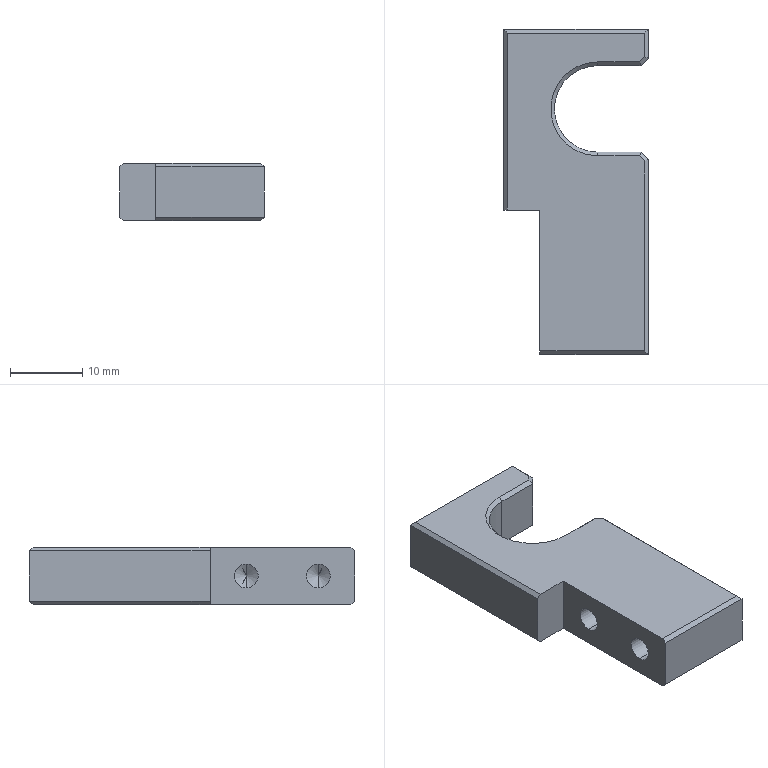Part | STEP file | PN_0063 Mount electronic clip s horizontal manipulator connecting rod | 1 solid | 43 faces | box 20 x 45 x 8 mm | volume 5111 mm3 | plane 31 | cone 7 | cylinder 5 | commonest cylinder face diameters 3.3 x4 12 x1